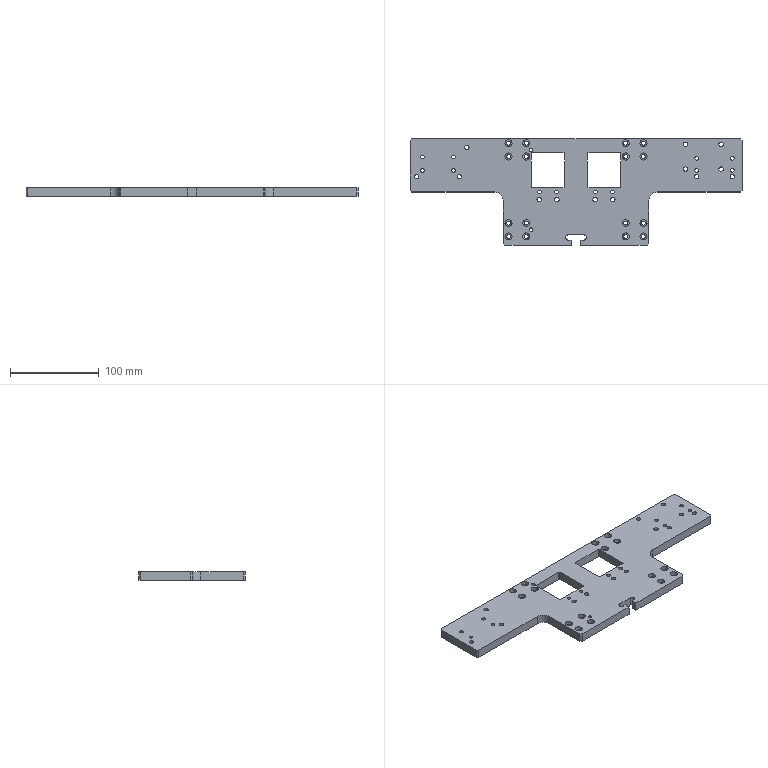CAM job | NX | 3-axis milling, drilling | part box 374 x 120 x 10 mm | stock box 379 x 125 x 10 mm
Tools:
number,name,description,diameter,corner_radius,flute_length,length,flutes
4,D4,平底铣刀-粗,4.0,0.0,25.0,75.0,2
9,D10,平底铣刀-粗,10.0,0.0,35.0,75.0,2
17,D2-J,平底铣刀-精,2.0,0.0,50.0,75.0,2
20,D3-J,平底铣刀-精,3.0,0.0,50.0,75.0,2
11,D4-J,平底铣刀-精,4.0,0.0,50.0,75.0,2
7,D6-J,平底铣刀-精,6.0,0.0,25.0,75.0,2
2,D6倒角刀,倒角刀,6.0,0.0,3.0,25.0,2
11,ZT4.5,钻头,4.5,0.0,35.0,50.0,2
18,ZT3.9,Drilling Tool,3.9,0.0,35.0,50.0,2
14,ZT4.3,Drilling Tool,4.3,0.0,50.0,75.0,4
19,ZT4.9,Drilling Tool,4.9,0.0,35.0,50.0,2
Operations:
program,operation,operation_type,tool,method,geometry_group,spindle_rpm,surface_speed,feed_per_tooth,feed_cut,feed_plunge,cut_length_mm,path_length_mm,cut_time_min,machine_time_min
B,C0.3_CONTOURCHAMFER6X45L_COPY,PlanarMilling,D6倒角刀,SLOPE_CHAMFER-DEPTH0-STEPG,W-B,7000.0,131.0,0.1071,1500.0,100.0,1354.034,1788.713,0.9027,0.9462
B,DRILLCHAMFER_4,Operation,D6倒角刀,METHOD,W-B,8000.0,150.796,0.0625,1000.0,0.0,10.6,214.25,0.0106,0.031
B,DRILLCHAMFER_5,Operation,D6倒角刀,METHOD,W-B,8000.0,150.796,0.0625,1000.0,0.0,88.8,788.032,0.0888,0.1587
B,DRILLCHAMFER_6,Operation,D6倒角刀,METHOD,W-B,8000.0,150.796,0.0625,1000.0,0.0,75.4,778.587,0.0754,0.1457
B,DRILLCHAMFER_7,Operation,D6倒角刀,METHOD,W-B,8000.0,150.796,0.0625,1000.0,0.0,68.4,683.985,0.0684,0.13
A,SPOTDRILL,Operation,D6倒角刀,METHOD,W-A,3000.0,56.549,0.0333,200.0,0.0,32.5,627.108,0.1625,0.222
A,SPOTDRILL_2,Operation,D6倒角刀,METHOD,W-A,3000.0,56.549,0.0333,200.0,0.0,75.0,1014.418,0.375,0.4689
A,PUNCHHOLE,Operation,ZT3.9,METHOD,W-A,3000.0,35.814,0.02,120.0,0.0,21.0,193.006,0.175,0.1922
A,PUNCHHOLE_2,Operation,ZT4.3,METHOD,W-A,3000.0,39.584,0.0167,100.0,0.0,126.0,735.269,1.26,1.321
A,PUNCHHOLE_4,Operation,ZT4.5,METHOD,W-A,2500.0,35.343,0.024,120.0,0.0,168.0,873.384,1.4,1.47
A,PUNCHHOLE_3,Operation,ZT4.9,METHOD,W-A,3000.0,45.239,0.025,150.0,0.0,136.5,835.108,0.91,0.9799
A,POCKETROUGH_1,VolumeBased25DMillingOperation,D10,METHOD,W-A,6000.0,188.0,0.25,4000.0,80.0,4757.444,4956.944,1.189,1.209
A,HOLEROUGH_1,CylinderMilling,D4,METHOD,W-A,6000.0,75.398,0.15,1800.0,100.0,3008.515,4504.315,1.671,1.821
A,CORNERCLEAN_D4,ZLevelMilling,D2-J,METHOD,W-A,6000.0,75.0,0.25,2500.0,80.0,3700.279,4176.162,1.481,1.529
A,PROFILEROUGH_2,VolumeBased25DMillingOperation,D10,METHOD,W-A,6000.0,188.0,0.25,4000.0,80.0,21501.773,21569.773,5.375,5.382
A,POCKETSEMI_1,VolumeBased25DMillingOperation,D6-J,METHOD,W-A,6000.0,113.0,0.0833,1000.0,100.0,270.083,489.384,0.2701,0.292
A,POCKETFINISH_1,VolumeBased25DMillingOperation,D6-J,METHOD,W-A,6000.0,113.0,0.0833,1000.0,100.0,269.683,490.283,0.2697,0.2917
A,HOLESIDE_1,CylinderMilling,D4-J,METHOD,W-A,6000.0,75.398,0.05,600.0,100.0,280.283,1854.483,0.4671,0.6246
A,PROFILED4_CORNER,ZLevelMilling,D4-J,METHOD,W-A,6000.0,75.0,0.25,2500.0,80.0,1489.12,1558.017,0.5958,0.6026
A,FLOORWALLSPIRALFINISH_MID_COPY_COPY_COPY_1_COPY,VolumeBased25DMillingOperation,D3-J,SPIRALFINISH-DEPTHK-STEPG,W-A,8000.0,50.266,0.0187,300.0,100.0,1106.999,2338.727,3.69,3.813
A,FLOORWALLSPIRALFINISH_MID_COPY_COPY_COPY_1_COPY_COPY,VolumeBased25DMillingOperation,D3-J,SPIRALFINISH-DEPTHK-STEPG,W-A,8000.0,50.266,0.0187,300.0,100.0,1099.143,2734.666,3.664,3.827
A,CHAMFER_2,SurfaceContour,D6倒角刀,METHOD,W-A,6000.0,113.0,0.125,1200.0,100.0,1337.624,1574.977,1.115,1.138
A,DRILLCHAMFER_1,Operation,D6倒角刀,METHOD,W-A,5000.0,94.248,0.015,150.0,0.0,10.6,174.25,0.0707,0.087
A,DRILLCHAMFER_2,Operation,D6倒角刀,METHOD,W-A,5000.0,94.248,0.015,150.0,0.0,75.4,738.587,0.5027,0.569
A,DRILLCHAMFER_3,Operation,D6倒角刀,METHOD,W-A,5000.0,94.248,0.015,150.0,0.0,68.4,643.985,0.456,0.5136
A,MILLCHAMFER_1,PlanarMilling,D6倒角刀,METHOD,W-A,6000.0,113.097,0.05,600.0,100.0,335.419,1805.967,0.559,0.7061
A,FLOORWALLSPIRALFINISH_MID_COPY_COPY_COPY,VolumeBased25DMillingOperation,D3-J,SPIRALFINISH-DEPTHK-STEPG,W-A,8000.0,50.266,0.0187,300.0,100.0,1882.142,3264.036,6.274,6.412
A,FLOORWALLSPIRALFINISH_MID_COPY_COPY_COPY_COPY,VolumeBased25DMillingOperation,D2-J,SPIRALFINISH-DEPTHK-STEPG,W-A,8000.0,50.266,0.0187,300.0,100.0,289.56,516.171,0.9652,0.9879
A,PROFILESEMI_2,VolumeBased25DMillingOperation,D6-J,METHOD,W-A,6000.0,113.0,0.0833,1000.0,100.0,1038.602,1116.602,1.039,1.046
A,PROFILEFINISH_2,VolumeBased25DMillingOperation,D6-J,METHOD,W-A,6000.0,113.0,0.0833,1000.0,100.0,1038.402,1117.002,1.038,1.046